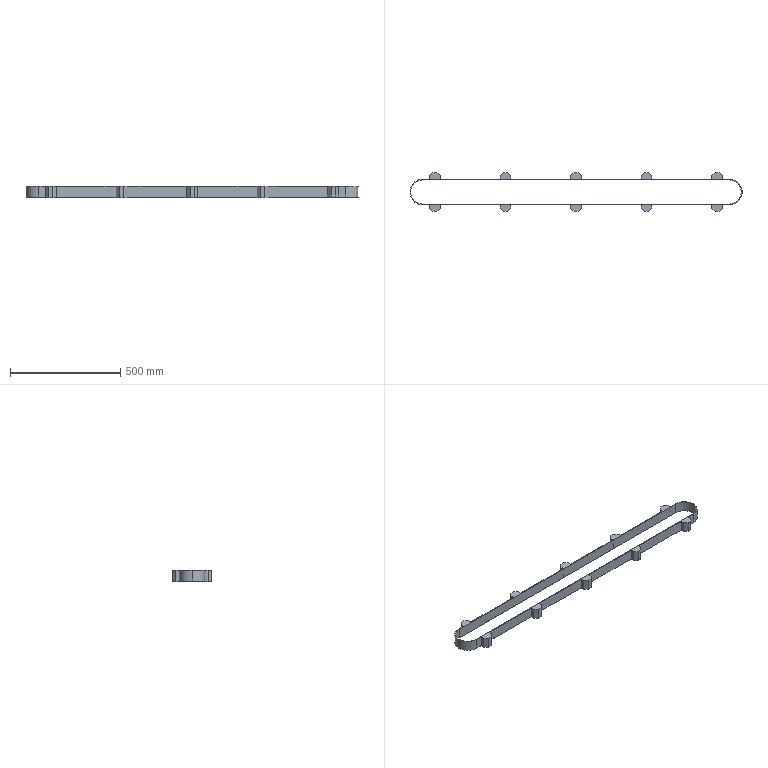Part | 1 solid | 88 faces | box 1506 x 176 x 50 mm | volume 1054080 mm3 | plane 82 | cylinder 6 | commonest cylinder face diameters 110 x3 116 x3